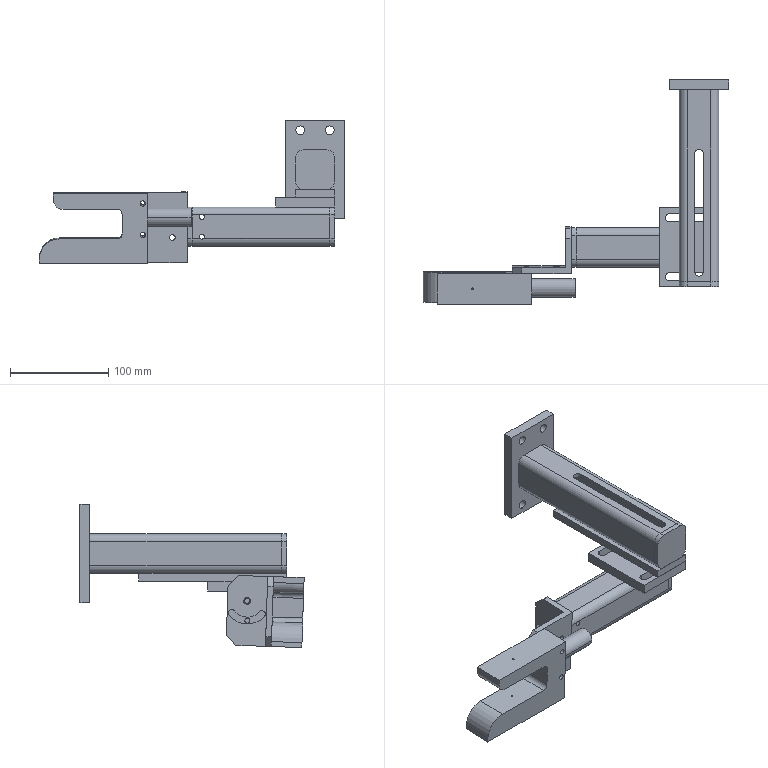Part | SolidWorks | 10 solids | 181 faces | box 310 x 227.812 x 145.36 mm | volume 532753 mm3 | cylinder 90 | plane 89 | cone 2 | commonest cylinder face diameters 16 x20 5 x14 9 x14 8 x8 7 x6 2 x4